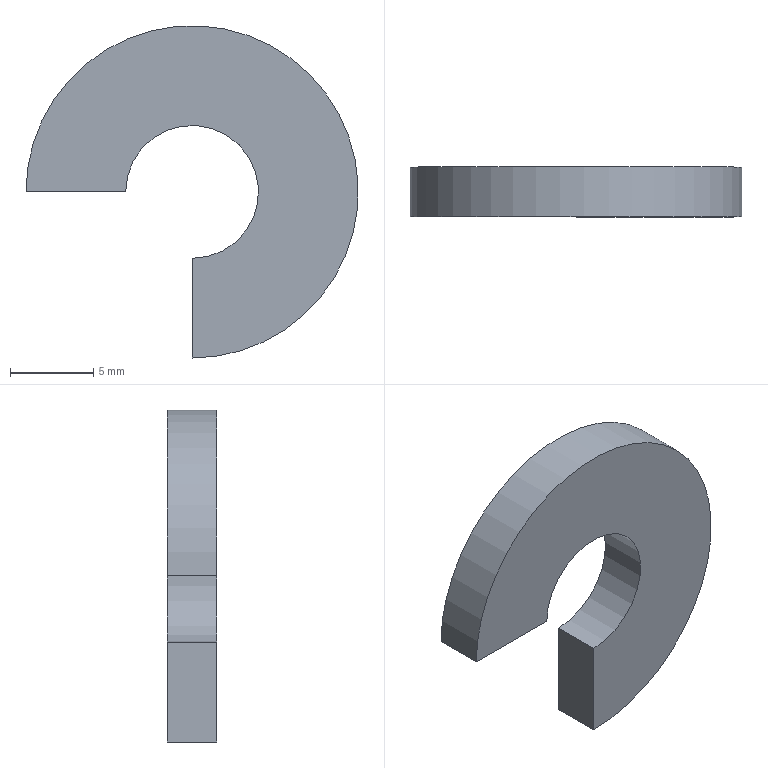Part | STEP file | Cuon T phu H01_8 | 1 solid | 6 faces | box 20 x 3 x 20 mm | volume 593.761 mm3 | plane 4 | cylinder 2 | commonest cylinder face diameters 8 x1 20 x1
STEP:
#1=CARTESIAN_POINT('',(0.,0.,0.));
#2=DIRECTION('',(0.,0.,1.));
#3=DIRECTION('',(1.,0.,0.));
#4=AXIS2_PLACEMENT_3D('',#1,#2,#3);
#5=CARTESIAN_POINT('',(-10.,3.,0.));
#6=VERTEX_POINT('',#5);
#7=CARTESIAN_POINT('',(-4.,3.,0.));
#8=VERTEX_POINT('',#7);
#9=CARTESIAN_POINT('',(0.,3.,0.));
#10=DIRECTION('',(1.,0.,0.));
#11=VECTOR('',#10,1.);
#12=LINE('',#9,#11);
#13=CARTESIAN_POINT('',(0.,3.,0.));
#14=DIRECTION('',(0.,1.,0.));
#15=DIRECTION('',(0.,0.,1.));
#16=AXIS2_PLACEMENT_3D('',#13,#14,#15);
#17=PLANE('',#16);
#18=CARTESIAN_POINT('',(0.,0.));
#19=DIRECTION('',(0.,1.));
#20=VECTOR('',#19,1.);
#21=LINE('',#18,#20);
#22=(GEOMETRIC_REPRESENTATION_CONTEXT(2)PARAMETRIC_REPRESENTATION_CONTEXT()REPRESENTATION_CONTEXT('',''));
#23=DEFINITIONAL_REPRESENTATION('',(#21),#22);
#24=PCURVE('',#17,#23);
#25=CARTESIAN_POINT('',(0.,-95.57,0.));
#26=DIRECTION('',(0.,0.,1.));
#27=DIRECTION('',(1.,0.,0.));
#28=AXIS2_PLACEMENT_3D('',#25,#26,#27);
#29=PLANE('',#28);
#30=CARTESIAN_POINT('',(0.,98.57));
#31=DIRECTION('',(1.,0.));
#32=VECTOR('',#31,1.);
#33=LINE('',#30,#32);
#34=(GEOMETRIC_REPRESENTATION_CONTEXT(2)PARAMETRIC_REPRESENTATION_CONTEXT()REPRESENTATION_CONTEXT('',''));
#35=DEFINITIONAL_REPRESENTATION('',(#33),#34);
#36=PCURVE('',#29,#35);
#37=SURFACE_CURVE('',#12,(#24,#36),.PCURVE_S1.);
#38=EDGE_CURVE('',#6,#8,#37,.T.);
#39=ORIENTED_EDGE('',*,*,#38,.F.);
#40=CARTESIAN_POINT('',(0.,3.,-10.));
#41=VERTEX_POINT('',#40);
#42=CARTESIAN_POINT('',(0.,3.,0.));
#43=DIRECTION('',(0.,1.,0.));
#44=DIRECTION('',(0.,0.,1.));
#45=AXIS2_PLACEMENT_3D('',#42,#43,#44);
#46=CIRCLE('',#45,10.);
#47=CARTESIAN_POINT('',(0.,0.));
#48=DIRECTION('',(1.,0.));
#49=AXIS2_PLACEMENT_2D('',#47,#48);
#50=CIRCLE('',#49,10.);
#51=(GEOMETRIC_REPRESENTATION_CONTEXT(2)PARAMETRIC_REPRESENTATION_CONTEXT()REPRESENTATION_CONTEXT('',''));
#52=DEFINITIONAL_REPRESENTATION('',(#50),#51);
#53=PCURVE('',#17,#52);
#54=CARTESIAN_POINT('',(0.,3.,0.));
#55=DIRECTION('',(0.,-1.,0.));
#56=DIRECTION('',(0.,0.,-1.));
#57=AXIS2_PLACEMENT_3D('',#54,#55,#56);
#58=CYLINDRICAL_SURFACE('',#57,10.);
#59=CARTESIAN_POINT('',(9.425,0.));
#60=DIRECTION('',(-1.,0.));
#61=VECTOR('',#60,1.);
#62=LINE('',#59,#61);
#63=(GEOMETRIC_REPRESENTATION_CONTEXT(2)PARAMETRIC_REPRESENTATION_CONTEXT()REPRESENTATION_CONTEXT('',''));
#64=DEFINITIONAL_REPRESENTATION('',(#62),#63);
#65=PCURVE('',#58,#64);
#66=SURFACE_CURVE('',#46,(#53,#65),.PCURVE_S1.);
#67=EDGE_CURVE('',#6,#41,#66,.T.);
#68=ORIENTED_EDGE('',*,*,#67,.T.);
#69=CARTESIAN_POINT('',(0.,3.,-4.));
#70=VERTEX_POINT('',#69);
#71=CARTESIAN_POINT('',(0.,3.,0.));
#72=DIRECTION('',(0.,0.,1.));
#73=VECTOR('',#72,1.);
#74=LINE('',#71,#73);
#75=CARTESIAN_POINT('',(0.,0.));
#76=DIRECTION('',(1.,0.));
#77=VECTOR('',#76,1.);
#78=LINE('',#75,#77);
#79=(GEOMETRIC_REPRESENTATION_CONTEXT(2)PARAMETRIC_REPRESENTATION_CONTEXT()REPRESENTATION_CONTEXT('',''));
#80=DEFINITIONAL_REPRESENTATION('',(#78),#79);
#81=PCURVE('',#17,#80);
#82=CARTESIAN_POINT('',(0.,-106.834,33.935));
#83=DIRECTION('',(-1.,0.,0.));
#84=DIRECTION('',(0.,0.,1.));
#85=AXIS2_PLACEMENT_3D('',#82,#83,#84);
#86=PLANE('',#85);
#87=CARTESIAN_POINT('',(-33.935,109.834));
#88=DIRECTION('',(1.,0.));
#89=VECTOR('',#88,1.);
#90=LINE('',#87,#89);
#91=(GEOMETRIC_REPRESENTATION_CONTEXT(2)PARAMETRIC_REPRESENTATION_CONTEXT()REPRESENTATION_CONTEXT('',''));
#92=DEFINITIONAL_REPRESENTATION('',(#90),#91);
#93=PCURVE('',#86,#92);
#94=SURFACE_CURVE('',#74,(#81,#93),.PCURVE_S1.);
#95=EDGE_CURVE('',#41,#70,#94,.T.);
#96=ORIENTED_EDGE('',*,*,#95,.T.);
#97=CARTESIAN_POINT('',(0.,3.,0.));
#98=DIRECTION('',(0.,1.,0.));
#99=DIRECTION('',(0.,0.,1.));
#100=AXIS2_PLACEMENT_3D('',#97,#98,#99);
#101=CIRCLE('',#100,4.);
#102=CARTESIAN_POINT('',(0.,0.));
#103=DIRECTION('',(1.,0.));
#104=AXIS2_PLACEMENT_2D('',#102,#103);
#105=CIRCLE('',#104,4.);
#106=(GEOMETRIC_REPRESENTATION_CONTEXT(2)PARAMETRIC_REPRESENTATION_CONTEXT()REPRESENTATION_CONTEXT('',''));
#107=DEFINITIONAL_REPRESENTATION('',(#105),#106);
#108=PCURVE('',#17,#107);
#109=CARTESIAN_POINT('',(0.,3.,0.));
#110=DIRECTION('',(0.,-1.,0.));
#111=DIRECTION('',(0.,0.,-1.));
#112=AXIS2_PLACEMENT_3D('',#109,#110,#111);
#113=CYLINDRICAL_SURFACE('',#112,4.);
#114=CARTESIAN_POINT('',(9.425,0.));
#115=DIRECTION('',(-1.,0.));
#116=VECTOR('',#115,1.);
#117=LINE('',#114,#116);
#118=(GEOMETRIC_REPRESENTATION_CONTEXT(2)PARAMETRIC_REPRESENTATION_CONTEXT()REPRESENTATION_CONTEXT('',''));
#119=DEFINITIONAL_REPRESENTATION('',(#117),#118);
#120=PCURVE('',#113,#119);
#121=SURFACE_CURVE('',#101,(#108,#120),.PCURVE_S1.);
#122=EDGE_CURVE('',#8,#70,#121,.T.);
#123=ORIENTED_EDGE('',*,*,#122,.F.);
#124=EDGE_LOOP('',(#39,#68,#96,#123));
#125=FACE_BOUND('',#124,.T.);
#126=ADVANCED_FACE('',(#125),#17,.T.);
#127=CARTESIAN_POINT('',(-10.,0.,0.));
#128=VERTEX_POINT('',#127);
#129=CARTESIAN_POINT('',(0.,0.,-10.));
#130=VERTEX_POINT('',#129);
#131=CARTESIAN_POINT('',(0.,0.,0.));
#132=DIRECTION('',(0.,1.,0.));
#133=DIRECTION('',(0.,0.,1.));
#134=AXIS2_PLACEMENT_3D('',#131,#132,#133);
#135=CIRCLE('',#134,10.);
#136=CARTESIAN_POINT('',(0.,0.,0.));
#137=DIRECTION('',(0.,1.,0.));
#138=DIRECTION('',(0.,0.,1.));
#139=AXIS2_PLACEMENT_3D('',#136,#137,#138);
#140=PLANE('',#139);
#141=CARTESIAN_POINT('',(0.,0.));
#142=DIRECTION('',(1.,0.));
#143=AXIS2_PLACEMENT_2D('',#141,#142);
#144=CIRCLE('',#143,10.);
#145=(GEOMETRIC_REPRESENTATION_CONTEXT(2)PARAMETRIC_REPRESENTATION_CONTEXT()REPRESENTATION_CONTEXT('',''));
#146=DEFINITIONAL_REPRESENTATION('',(#144),#145);
#147=PCURVE('',#140,#146);
#148=CARTESIAN_POINT('',(9.425,3.));
#149=DIRECTION('',(-1.,0.));
#150=VECTOR('',#149,1.);
#151=LINE('',#148,#150);
#152=(GEOMETRIC_REPRESENTATION_CONTEXT(2)PARAMETRIC_REPRESENTATION_CONTEXT()REPRESENTATION_CONTEXT('',''));
#153=DEFINITIONAL_REPRESENTATION('',(#151),#152);
#154=PCURVE('',#58,#153);
#155=SURFACE_CURVE('',#135,(#147,#154),.PCURVE_S1.);
#156=EDGE_CURVE('',#128,#130,#155,.T.);
#157=ORIENTED_EDGE('',*,*,#156,.F.);
#158=CARTESIAN_POINT('',(-4.,0.,0.));
#159=VERTEX_POINT('',#158);
#160=CARTESIAN_POINT('',(0.,0.,0.));
#161=DIRECTION('',(1.,0.,0.));
#162=VECTOR('',#161,1.);
#163=LINE('',#160,#162);
#164=CARTESIAN_POINT('',(0.,0.));
#165=DIRECTION('',(0.,1.));
#166=VECTOR('',#165,1.);
#167=LINE('',#164,#166);
#168=(GEOMETRIC_REPRESENTATION_CONTEXT(2)PARAMETRIC_REPRESENTATION_CONTEXT()REPRESENTATION_CONTEXT('',''));
#169=DEFINITIONAL_REPRESENTATION('',(#167),#168);
#170=PCURVE('',#140,#169);
#171=CARTESIAN_POINT('',(0.,95.57));
#172=DIRECTION('',(1.,0.));
#173=VECTOR('',#172,1.);
#174=LINE('',#171,#173);
#175=(GEOMETRIC_REPRESENTATION_CONTEXT(2)PARAMETRIC_REPRESENTATION_CONTEXT()REPRESENTATION_CONTEXT('',''));
#176=DEFINITIONAL_REPRESENTATION('',(#174),#175);
#177=PCURVE('',#29,#176);
#178=SURFACE_CURVE('',#163,(#170,#177),.PCURVE_S1.);
#179=EDGE_CURVE('',#128,#159,#178,.T.);
#180=ORIENTED_EDGE('',*,*,#179,.T.);
#181=CARTESIAN_POINT('',(0.,0.,-4.));
#182=VERTEX_POINT('',#181);
#183=CARTESIAN_POINT('',(0.,0.,0.));
#184=DIRECTION('',(0.,1.,0.));
#185=DIRECTION('',(0.,0.,1.));
#186=AXIS2_PLACEMENT_3D('',#183,#184,#185);
#187=CIRCLE('',#186,4.);
#188=CARTESIAN_POINT('',(0.,0.));
#189=DIRECTION('',(1.,0.));
#190=AXIS2_PLACEMENT_2D('',#188,#189);
#191=CIRCLE('',#190,4.);
#192=(GEOMETRIC_REPRESENTATION_CONTEXT(2)PARAMETRIC_REPRESENTATION_CONTEXT()REPRESENTATION_CONTEXT('',''));
#193=DEFINITIONAL_REPRESENTATION('',(#191),#192);
#194=PCURVE('',#140,#193);
#195=CARTESIAN_POINT('',(9.425,3.));
#196=DIRECTION('',(-1.,0.));
#197=VECTOR('',#196,1.);
#198=LINE('',#195,#197);
#199=(GEOMETRIC_REPRESENTATION_CONTEXT(2)PARAMETRIC_REPRESENTATION_CONTEXT()REPRESENTATION_CONTEXT('',''));
#200=DEFINITIONAL_REPRESENTATION('',(#198),#199);
#201=PCURVE('',#113,#200);
#202=SURFACE_CURVE('',#187,(#194,#201),.PCURVE_S1.);
#203=EDGE_CURVE('',#159,#182,#202,.T.);
#204=ORIENTED_EDGE('',*,*,#203,.T.);
#205=CARTESIAN_POINT('',(0.,0.,0.));
#206=DIRECTION('',(0.,0.,1.));
#207=VECTOR('',#206,1.);
#208=LINE('',#205,#207);
#209=CARTESIAN_POINT('',(0.,0.));
#210=DIRECTION('',(1.,0.));
#211=VECTOR('',#210,1.);
#212=LINE('',#209,#211);
#213=(GEOMETRIC_REPRESENTATION_CONTEXT(2)PARAMETRIC_REPRESENTATION_CONTEXT()REPRESENTATION_CONTEXT('',''));
#214=DEFINITIONAL_REPRESENTATION('',(#212),#213);
#215=PCURVE('',#140,#214);
#216=CARTESIAN_POINT('',(-33.935,106.834));
#217=DIRECTION('',(1.,0.));
#218=VECTOR('',#217,1.);
#219=LINE('',#216,#218);
#220=(GEOMETRIC_REPRESENTATION_CONTEXT(2)PARAMETRIC_REPRESENTATION_CONTEXT()REPRESENTATION_CONTEXT('',''));
#221=DEFINITIONAL_REPRESENTATION('',(#219),#220);
#222=PCURVE('',#86,#221);
#223=SURFACE_CURVE('',#208,(#215,#222),.PCURVE_S1.);
#224=EDGE_CURVE('',#130,#182,#223,.T.);
#225=ORIENTED_EDGE('',*,*,#224,.F.);
#226=EDGE_LOOP('',(#157,#180,#204,#225));
#227=FACE_BOUND('',#226,.T.);
#228=ADVANCED_FACE('',(#227),#140,.F.);
#229=ORIENTED_EDGE('',*,*,#67,.F.);
#230=CARTESIAN_POINT('',(-10.,3.,0.));
#231=DIRECTION('',(0.,-1.,0.));
#232=VECTOR('',#231,1.);
#233=LINE('',#230,#232);
#234=CARTESIAN_POINT('',(4.712,0.));
#235=DIRECTION('',(0.,1.));
#236=VECTOR('',#235,1.);
#237=LINE('',#234,#236);
#238=(GEOMETRIC_REPRESENTATION_CONTEXT(2)PARAMETRIC_REPRESENTATION_CONTEXT()REPRESENTATION_CONTEXT('',''));
#239=DEFINITIONAL_REPRESENTATION('',(#237),#238);
#240=PCURVE('',#58,#239);
#241=CARTESIAN_POINT('',(-10.,98.57));
#242=DIRECTION('',(0.,-1.));
#243=VECTOR('',#242,1.);
#244=LINE('',#241,#243);
#245=(GEOMETRIC_REPRESENTATION_CONTEXT(2)PARAMETRIC_REPRESENTATION_CONTEXT()REPRESENTATION_CONTEXT('',''));
#246=DEFINITIONAL_REPRESENTATION('',(#244),#245);
#247=PCURVE('',#29,#246);
#248=SURFACE_CURVE('',#233,(#240,#247),.PCURVE_S1.);
#249=EDGE_CURVE('',#6,#128,#248,.T.);
#250=ORIENTED_EDGE('',*,*,#249,.T.);
#251=ORIENTED_EDGE('',*,*,#156,.T.);
#252=CARTESIAN_POINT('',(0.,3.,-10.));
#253=DIRECTION('',(0.,-1.,0.));
#254=VECTOR('',#253,1.);
#255=LINE('',#252,#254);
#256=CARTESIAN_POINT('',(0.,0.));
#257=DIRECTION('',(0.,1.));
#258=VECTOR('',#257,1.);
#259=LINE('',#256,#258);
#260=(GEOMETRIC_REPRESENTATION_CONTEXT(2)PARAMETRIC_REPRESENTATION_CONTEXT()REPRESENTATION_CONTEXT('',''));
#261=DEFINITIONAL_REPRESENTATION('',(#259),#260);
#262=PCURVE('',#58,#261);
#263=CARTESIAN_POINT('',(-43.935,109.834));
#264=DIRECTION('',(0.,-1.));
#265=VECTOR('',#264,1.);
#266=LINE('',#263,#265);
#267=(GEOMETRIC_REPRESENTATION_CONTEXT(2)PARAMETRIC_REPRESENTATION_CONTEXT()REPRESENTATION_CONTEXT('',''));
#268=DEFINITIONAL_REPRESENTATION('',(#266),#267);
#269=PCURVE('',#86,#268);
#270=SURFACE_CURVE('',#255,(#262,#269),.PCURVE_S1.);
#271=EDGE_CURVE('',#41,#130,#270,.T.);
#272=ORIENTED_EDGE('',*,*,#271,.F.);
#273=EDGE_LOOP('',(#229,#250,#251,#272));
#274=FACE_BOUND('',#273,.T.);
#275=ADVANCED_FACE('',(#274),#58,.T.);
#276=ORIENTED_EDGE('',*,*,#203,.T.);
#277=CARTESIAN_POINT('',(0.,3.,-4.));
#278=DIRECTION('',(0.,-1.,0.));
#279=VECTOR('',#278,1.);
#280=LINE('',#277,#279);
#281=CARTESIAN_POINT('',(0.,0.));
#282=DIRECTION('',(0.,1.));
#283=VECTOR('',#282,1.);
#284=LINE('',#281,#283);
#285=(GEOMETRIC_REPRESENTATION_CONTEXT(2)PARAMETRIC_REPRESENTATION_CONTEXT()REPRESENTATION_CONTEXT('',''));
#286=DEFINITIONAL_REPRESENTATION('',(#284),#285);
#287=PCURVE('',#113,#286);
#288=CARTESIAN_POINT('',(-37.935,109.834));
#289=DIRECTION('',(0.,-1.));
#290=VECTOR('',#289,1.);
#291=LINE('',#288,#290);
#292=(GEOMETRIC_REPRESENTATION_CONTEXT(2)PARAMETRIC_REPRESENTATION_CONTEXT()REPRESENTATION_CONTEXT('',''));
#293=DEFINITIONAL_REPRESENTATION('',(#291),#292);
#294=PCURVE('',#86,#293);
#295=SURFACE_CURVE('',#280,(#287,#294),.PCURVE_S1.);
#296=EDGE_CURVE('',#70,#182,#295,.T.);
#297=ORIENTED_EDGE('',*,*,#296,.F.);
#298=ORIENTED_EDGE('',*,*,#122,.F.);
#299=CARTESIAN_POINT('',(-4.,3.,0.));
#300=DIRECTION('',(0.,-1.,0.));
#301=VECTOR('',#300,1.);
#302=LINE('',#299,#301);
#303=CARTESIAN_POINT('',(4.712,0.));
#304=DIRECTION('',(0.,1.));
#305=VECTOR('',#304,1.);
#306=LINE('',#303,#305);
#307=(GEOMETRIC_REPRESENTATION_CONTEXT(2)PARAMETRIC_REPRESENTATION_CONTEXT()REPRESENTATION_CONTEXT('',''));
#308=DEFINITIONAL_REPRESENTATION('',(#306),#307);
#309=PCURVE('',#113,#308);
#310=CARTESIAN_POINT('',(-4.,98.57));
#311=DIRECTION('',(0.,-1.));
#312=VECTOR('',#311,1.);
#313=LINE('',#310,#312);
#314=(GEOMETRIC_REPRESENTATION_CONTEXT(2)PARAMETRIC_REPRESENTATION_CONTEXT()REPRESENTATION_CONTEXT('',''));
#315=DEFINITIONAL_REPRESENTATION('',(#313),#314);
#316=PCURVE('',#29,#315);
#317=SURFACE_CURVE('',#302,(#309,#316),.PCURVE_S1.);
#318=EDGE_CURVE('',#8,#159,#317,.T.);
#319=ORIENTED_EDGE('',*,*,#318,.T.);
#320=EDGE_LOOP('',(#276,#297,#298,#319));
#321=FACE_BOUND('',#320,.F.);
#322=ADVANCED_FACE('',(#321),#113,.F.);
#323=ORIENTED_EDGE('',*,*,#271,.T.);
#324=ORIENTED_EDGE('',*,*,#224,.T.);
#325=ORIENTED_EDGE('',*,*,#296,.F.);
#326=ORIENTED_EDGE('',*,*,#95,.F.);
#327=EDGE_LOOP('',(#323,#324,#325,#326));
#328=FACE_BOUND('',#327,.T.);
#329=ADVANCED_FACE('',(#328),#86,.T.);
#330=ORIENTED_EDGE('',*,*,#38,.T.);
#331=ORIENTED_EDGE('',*,*,#318,.T.);
#332=ORIENTED_EDGE('',*,*,#179,.F.);
#333=ORIENTED_EDGE('',*,*,#249,.F.);
#334=EDGE_LOOP('',(#330,#331,#332,#333));
#335=FACE_BOUND('',#334,.T.);
#336=ADVANCED_FACE('',(#335),#29,.F.);
#337=CLOSED_SHELL('',(#126,#228,#275,#322,#329,#336));
#338=MANIFOLD_SOLID_BREP('',#337);
#339=(LENGTH_UNIT()NAMED_UNIT(*)SI_UNIT(.MILLI.,.METRE.));
#340=UNCERTAINTY_MEASURE_WITH_UNIT(LENGTH_MEASURE(0.0000001),#339,'','');
#341=(NAMED_UNIT(*)PLANE_ANGLE_UNIT()SI_UNIT($,.RADIAN.));
#342=(NAMED_UNIT(*)SI_UNIT($,.STERADIAN.)SOLID_ANGLE_UNIT());
#343=(GEOMETRIC_REPRESENTATION_CONTEXT(3)GLOBAL_UNCERTAINTY_ASSIGNED_CONTEXT((#340))GLOBAL_UNIT_ASSIGNED_CONTEXT((#339,#341,#342))REPRESENTATION_CONTEXT('',''));
#344=ADVANCED_BREP_SHAPE_REPRESENTATION('',(#4,#338),#343);